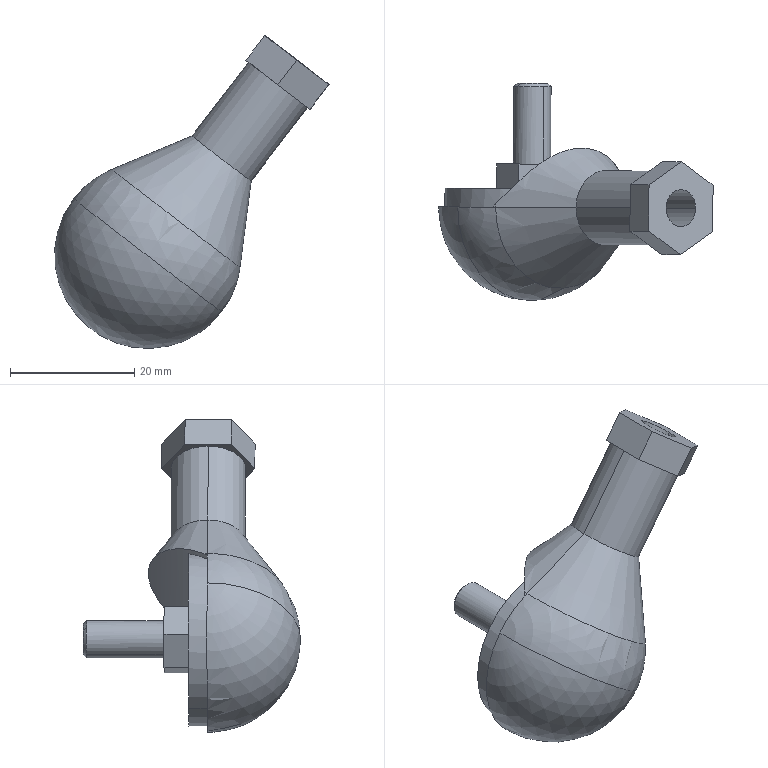Part | STEP file | 46B-01002ZX30 | 1 solid | 36 faces | box 44.236 x 35.015 x 50.429 mm | volume 13200 mm3 | plane 19 | cylinder 9 | cone 4 | sphere 4 | commonest cylinder face diameters 6 x4 12 x2 28 x2 72 x1